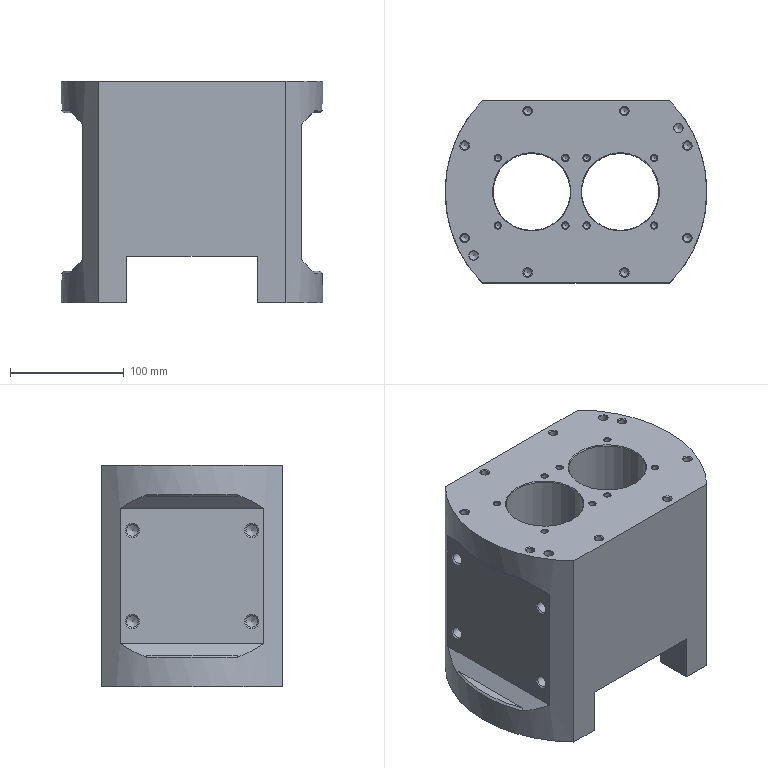Part | 1 solid | 154 faces | box 230 x 160 x 195 mm | volume 4011629 mm3 | cone 88 | cylinder 46 | plane 20 | commonest cylinder face diameters 5 x16 6.8 x8 10.2 x8 8.5 x4 8 x2 12 x2